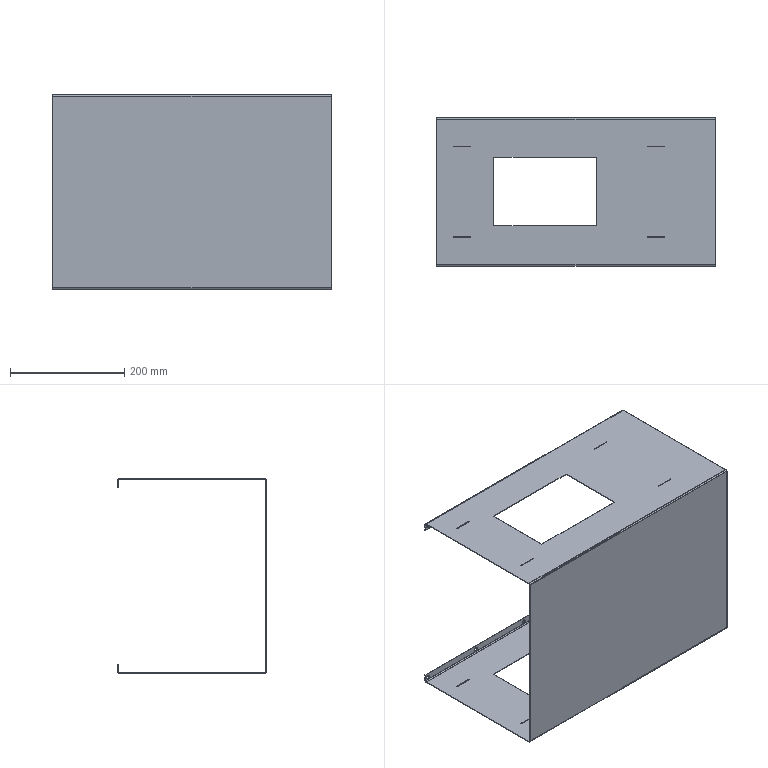Part | SolidWorks | features ICE 2, Cut 1, FlatPattern 1, MirrorPattern 1, SMBaseFlange 1, SheetMetal 1 | 1 solid | 98 faces | box 487.6 x 260 x 340 mm | volume 463191 mm3 | plane 70 | cylinder 28 | commonest cylinder face diameters 7 x20 3 x4 5.4 x4